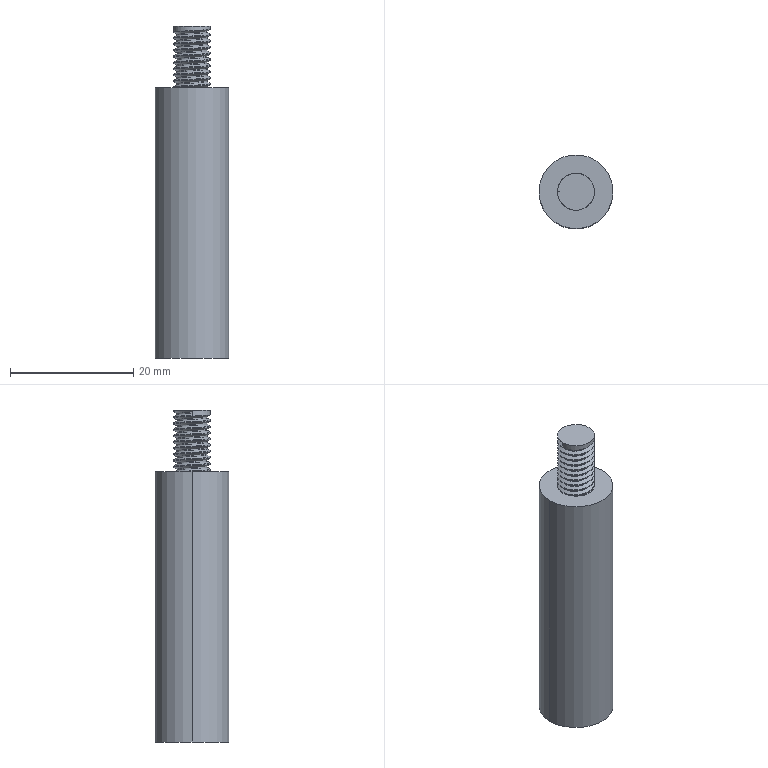Part | NX | features BREP 1 | 1 solid | 36 faces | box 12 x 12 x 53.85 mm | volume 5098 mm3 | cylinder 27 | plane 5 | cone 2 | spline 2 | commonest cylinder face diameters 6 x22 3.3 x2 12 x2 4.917 x1